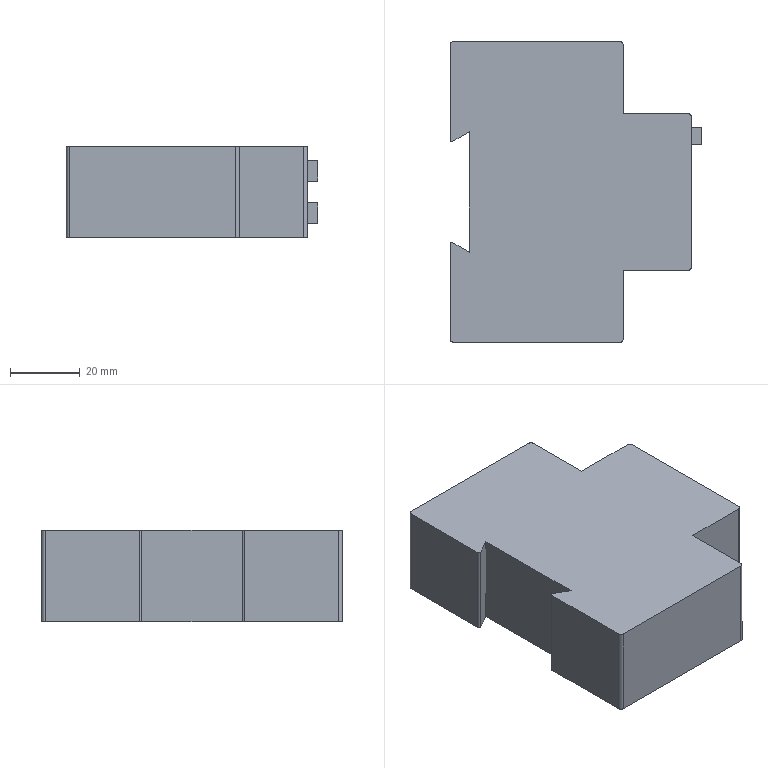Part | STEP file | _X2_52079664_X0_-_X2_62C94F38_X | 1 solid | 62 faces | box 71.959 x 86 x 26.2 mm | volume 129810 mm3 | plane 38 | cylinder 24 | commonest cylinder face diameters 4.125 x8 2 x6 3 x4 4 x4 1 x2